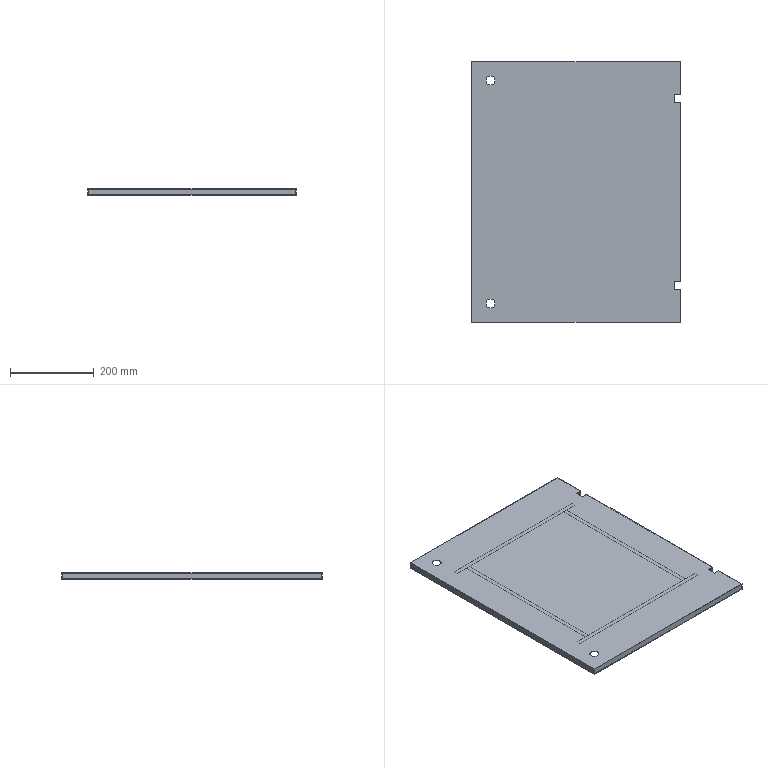Part | STEP file | 5 solids | 78 faces | box 498 x 622 x 16 mm | volume 475643 mm3 | plane 70 | cylinder 8 | commonest cylinder face diameters 22 x8